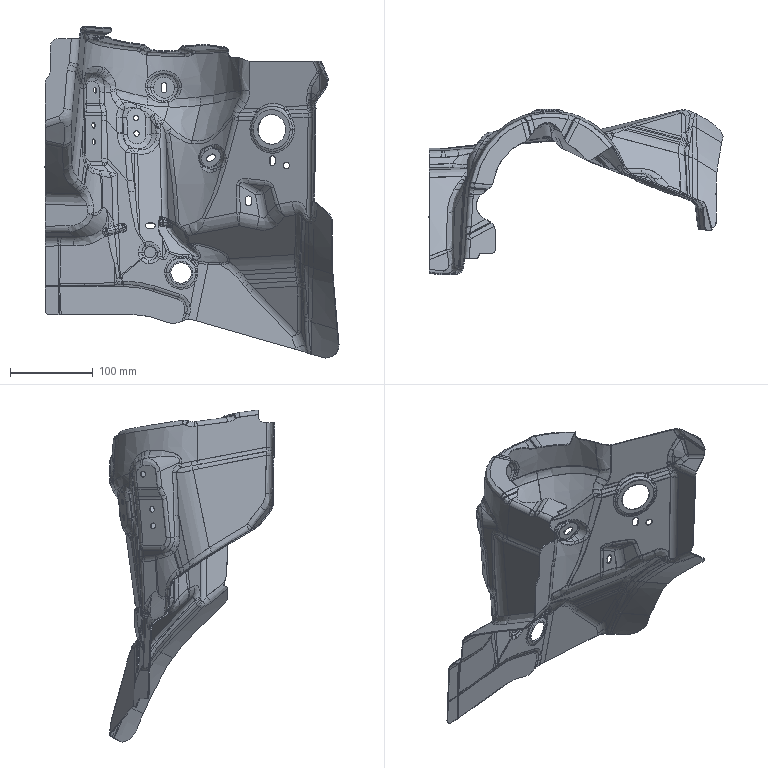Part | 1 solid | 1368 faces | box 355.654 x 199.978 x 401.521 mm | volume 194029 mm3 | spline 1051 | cylinder 194 | plane 107 | sphere 12 | other 4 | commonest cylinder face diameters 20 x27 17.6 x21 7 x20 24 x14 30 x14 27.6 x11